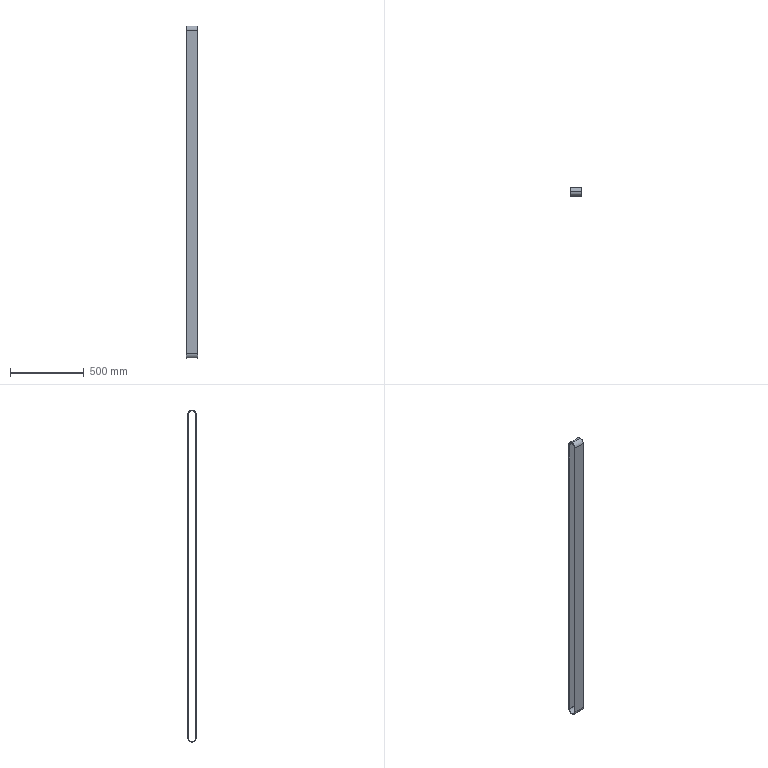Part | SolidWorks | features BossThin 1, ExtruThin 1 | 2 solids | 24 faces | box 80 x 59.15 x 2252 mm | volume 1851098 mm3 | cylinder 12 | plane 12 | commonest cylinder face diameters 54.65 x6 48.99 x3 59.15 x3
STEP:
#1=CARTESIAN_POINT('',(40.,27.325,0.));
#2=VERTEX_POINT('',#1);
#3=CARTESIAN_POINT('',(40.,0.,27.325));
#4=VERTEX_POINT('',#3);
#5=CARTESIAN_POINT('',(40.,0.,0.));
#6=DIRECTION('',(1.,0.,0.));
#7=DIRECTION('',(0.,0.,-1.));
#8=AXIS2_PLACEMENT_3D('',#5,#6,#7);
#9=CIRCLE('',#8,27.325);
#10=EDGE_CURVE('',#2,#4,#9,.T.);
#11=ORIENTED_EDGE('',*,*,#10,.T.);
#12=CARTESIAN_POINT('',(-40.,0.,27.325));
#13=VERTEX_POINT('',#12);
#14=CARTESIAN_POINT('',(40.,0.,27.325));
#15=DIRECTION('',(-1.,0.,0.));
#16=VECTOR('',#15,1000.);
#17=LINE('',#14,#16);
#18=EDGE_CURVE('',#4,#13,#17,.T.);
#19=ORIENTED_EDGE('',*,*,#18,.T.);
#20=CARTESIAN_POINT('',(-40.,27.325,0.));
#21=VERTEX_POINT('',#20);
#22=CARTESIAN_POINT('',(-40.,0.,0.));
#23=DIRECTION('',(1.,0.,0.));
#24=DIRECTION('',(0.,0.,-1.));
#25=AXIS2_PLACEMENT_3D('',#22,#23,#24);
#26=CIRCLE('',#25,27.325);
#27=EDGE_CURVE('',#21,#13,#26,.T.);
#28=ORIENTED_EDGE('',*,*,#27,.F.);
#29=CARTESIAN_POINT('',(40.,27.325,0.));
#30=DIRECTION('',(-1.,0.,0.));
#31=VECTOR('',#30,1000.);
#32=LINE('',#29,#31);
#33=EDGE_CURVE('',#2,#21,#32,.T.);
#34=ORIENTED_EDGE('',*,*,#33,.F.);
#35=EDGE_LOOP('',(#11,#19,#28,#34));
#36=FACE_OUTER_BOUND('',#35,.T.);
#37=CARTESIAN_POINT('',(40.,0.,0.));
#38=DIRECTION('',(-1.,0.,0.));
#39=DIRECTION('',(0.,0.,1.));
#40=AXIS2_PLACEMENT_3D('',#37,#38,#39);
#41=CYLINDRICAL_SURFACE('',#40,27.325);
#42=ADVANCED_FACE('',(#36),#41,.F.);
#43=CARTESIAN_POINT('',(40.,0.,29.575));
#44=VERTEX_POINT('',#43);
#45=CARTESIAN_POINT('',(40.,-29.575,0.));
#46=VERTEX_POINT('',#45);
#47=CARTESIAN_POINT('',(40.,0.,0.));
#48=DIRECTION('',(1.,0.,0.));
#49=DIRECTION('',(0.,0.,-1.));
#50=AXIS2_PLACEMENT_3D('',#47,#48,#49);
#51=CIRCLE('',#50,29.575);
#52=EDGE_CURVE('',#44,#46,#51,.T.);
#53=ORIENTED_EDGE('',*,*,#52,.F.);
#54=CARTESIAN_POINT('',(-40.,0.,29.575));
#55=VERTEX_POINT('',#54);
#56=CARTESIAN_POINT('',(40.,0.,29.575));
#57=DIRECTION('',(-1.,0.,0.));
#58=VECTOR('',#57,1000.);
#59=LINE('',#56,#58);
#60=EDGE_CURVE('',#44,#55,#59,.T.);
#61=ORIENTED_EDGE('',*,*,#60,.T.);
#62=CARTESIAN_POINT('',(-40.,-29.575,0.));
#63=VERTEX_POINT('',#62);
#64=CARTESIAN_POINT('',(-40.,0.,0.));
#65=DIRECTION('',(1.,0.,0.));
#66=DIRECTION('',(0.,0.,-1.));
#67=AXIS2_PLACEMENT_3D('',#64,#65,#66);
#68=CIRCLE('',#67,29.575);
#69=EDGE_CURVE('',#55,#63,#68,.T.);
#70=ORIENTED_EDGE('',*,*,#69,.T.);
#71=CARTESIAN_POINT('',(40.,-29.575,0.));
#72=DIRECTION('',(-1.,0.,0.));
#73=VECTOR('',#72,1000.);
#74=LINE('',#71,#73);
#75=EDGE_CURVE('',#46,#63,#74,.T.);
#76=ORIENTED_EDGE('',*,*,#75,.F.);
#77=EDGE_LOOP('',(#53,#61,#70,#76));
#78=FACE_OUTER_BOUND('',#77,.T.);
#79=CARTESIAN_POINT('',(40.,0.,0.));
#80=DIRECTION('',(-1.,0.,0.));
#81=DIRECTION('',(0.,0.,1.));
#82=AXIS2_PLACEMENT_3D('',#79,#80,#81);
#83=CYLINDRICAL_SURFACE('',#82,29.575);
#84=ADVANCED_FACE('',(#78),#83,.T.);
#85=CARTESIAN_POINT('',(40.,29.575,0.));
#86=VERTEX_POINT('',#85);
#87=CARTESIAN_POINT('',(40.,0.,0.));
#88=DIRECTION('',(1.,0.,0.));
#89=DIRECTION('',(0.,0.,-1.));
#90=AXIS2_PLACEMENT_3D('',#87,#88,#89);
#91=CIRCLE('',#90,29.575);
#92=EDGE_CURVE('',#86,#44,#91,.T.);
#93=ORIENTED_EDGE('',*,*,#92,.T.);
#94=ORIENTED_EDGE('',*,*,#52,.T.);
#95=CARTESIAN_POINT('',(40.,-29.575,-2192.5));
#96=VERTEX_POINT('',#95);
#97=CARTESIAN_POINT('',(40.,-29.575,0.));
#98=DIRECTION('',(0.,0.,-1.));
#99=VECTOR('',#98,1000.);
#100=LINE('',#97,#99);
#101=EDGE_CURVE('',#46,#96,#100,.T.);
#102=ORIENTED_EDGE('',*,*,#101,.T.);
#103=CARTESIAN_POINT('',(40.,29.575,-2192.5));
#104=VERTEX_POINT('',#103);
#105=CARTESIAN_POINT('',(40.,0.,-2192.5));
#106=DIRECTION('',(1.,0.,0.));
#107=DIRECTION('',(0.,0.,-1.));
#108=AXIS2_PLACEMENT_3D('',#105,#106,#107);
#109=CIRCLE('',#108,29.575);
#110=EDGE_CURVE('',#96,#104,#109,.T.);
#111=ORIENTED_EDGE('',*,*,#110,.T.);
#112=CARTESIAN_POINT('',(40.,29.575,0.));
#113=DIRECTION('',(0.,0.,1.));
#114=VECTOR('',#113,1000.);
#115=LINE('',#112,#114);
#116=EDGE_CURVE('',#104,#86,#115,.T.);
#117=ORIENTED_EDGE('',*,*,#116,.T.);
#118=EDGE_LOOP('',(#93,#94,#102,#111,#117));
#119=FACE_OUTER_BOUND('',#118,.T.);
#120=CARTESIAN_POINT('',(40.,-27.325,0.));
#121=VERTEX_POINT('',#120);
#122=CARTESIAN_POINT('',(40.,-27.325,-2192.5));
#123=VERTEX_POINT('',#122);
#124=CARTESIAN_POINT('',(40.,-27.325,0.));
#125=DIRECTION('',(0.,0.,-1.));
#126=VECTOR('',#125,1000.);
#127=LINE('',#124,#126);
#128=EDGE_CURVE('',#121,#123,#127,.T.);
#129=ORIENTED_EDGE('',*,*,#128,.F.);
#130=CARTESIAN_POINT('',(40.,0.,0.));
#131=DIRECTION('',(1.,0.,0.));
#132=DIRECTION('',(0.,0.,-1.));
#133=AXIS2_PLACEMENT_3D('',#130,#131,#132);
#134=CIRCLE('',#133,27.325);
#135=EDGE_CURVE('',#4,#121,#134,.T.);
#136=ORIENTED_EDGE('',*,*,#135,.F.);
#137=ORIENTED_EDGE('',*,*,#10,.F.);
#138=CARTESIAN_POINT('',(40.,27.325,-2192.5));
#139=VERTEX_POINT('',#138);
#140=CARTESIAN_POINT('',(40.,27.325,0.));
#141=DIRECTION('',(0.,0.,1.));
#142=VECTOR('',#141,1000.);
#143=LINE('',#140,#142);
#144=EDGE_CURVE('',#139,#2,#143,.T.);
#145=ORIENTED_EDGE('',*,*,#144,.F.);
#146=CARTESIAN_POINT('',(40.,0.,-2192.5));
#147=DIRECTION('',(1.,0.,0.));
#148=DIRECTION('',(0.,0.,-1.));
#149=AXIS2_PLACEMENT_3D('',#146,#147,#148);
#150=CIRCLE('',#149,27.325);
#151=EDGE_CURVE('',#123,#139,#150,.T.);
#152=ORIENTED_EDGE('',*,*,#151,.F.);
#153=EDGE_LOOP('',(#129,#136,#137,#145,#152));
#154=FACE_BOUND('',#153,.T.);
#155=CARTESIAN_POINT('',(40.,0.,0.));
#156=DIRECTION('',(1.,0.,0.));
#157=DIRECTION('',(0.,0.,-1.));
#158=AXIS2_PLACEMENT_3D('',#155,#156,#157);
#159=PLANE('',#158);
#160=ADVANCED_FACE('',(#119,#154),#159,.T.);
#161=CARTESIAN_POINT('',(-40.,29.575,0.));
#162=VERTEX_POINT('',#161);
#163=CARTESIAN_POINT('',(-40.,0.,0.));
#164=DIRECTION('',(1.,0.,0.));
#165=DIRECTION('',(0.,0.,-1.));
#166=AXIS2_PLACEMENT_3D('',#163,#164,#165);
#167=CIRCLE('',#166,29.575);
#168=EDGE_CURVE('',#162,#55,#167,.T.);
#169=ORIENTED_EDGE('',*,*,#168,.F.);
#170=CARTESIAN_POINT('',(-40.,29.575,-2192.5));
#171=VERTEX_POINT('',#170);
#172=CARTESIAN_POINT('',(-40.,29.575,0.));
#173=DIRECTION('',(0.,0.,1.));
#174=VECTOR('',#173,1000.);
#175=LINE('',#172,#174);
#176=EDGE_CURVE('',#171,#162,#175,.T.);
#177=ORIENTED_EDGE('',*,*,#176,.F.);
#178=CARTESIAN_POINT('',(-40.,-29.575,-2192.5));
#179=VERTEX_POINT('',#178);
#180=CARTESIAN_POINT('',(-40.,0.,-2192.5));
#181=DIRECTION('',(1.,0.,0.));
#182=DIRECTION('',(0.,0.,-1.));
#183=AXIS2_PLACEMENT_3D('',#180,#181,#182);
#184=CIRCLE('',#183,29.575);
#185=EDGE_CURVE('',#179,#171,#184,.T.);
#186=ORIENTED_EDGE('',*,*,#185,.F.);
#187=CARTESIAN_POINT('',(-40.,-29.575,0.));
#188=DIRECTION('',(0.,0.,-1.));
#189=VECTOR('',#188,1000.);
#190=LINE('',#187,#189);
#191=EDGE_CURVE('',#63,#179,#190,.T.);
#192=ORIENTED_EDGE('',*,*,#191,.F.);
#193=ORIENTED_EDGE('',*,*,#69,.F.);
#194=EDGE_LOOP('',(#169,#177,#186,#192,#193));
#195=FACE_OUTER_BOUND('',#194,.T.);
#196=ORIENTED_EDGE('',*,*,#27,.T.);
#197=CARTESIAN_POINT('',(-40.,-27.325,0.));
#198=VERTEX_POINT('',#197);
#199=CARTESIAN_POINT('',(-40.,0.,0.));
#200=DIRECTION('',(1.,0.,0.));
#201=DIRECTION('',(0.,0.,-1.));
#202=AXIS2_PLACEMENT_3D('',#199,#200,#201);
#203=CIRCLE('',#202,27.325);
#204=EDGE_CURVE('',#13,#198,#203,.T.);
#205=ORIENTED_EDGE('',*,*,#204,.T.);
#206=CARTESIAN_POINT('',(-40.,-27.325,-2192.5));
#207=VERTEX_POINT('',#206);
#208=CARTESIAN_POINT('',(-40.,-27.325,0.));
#209=DIRECTION('',(0.,0.,-1.));
#210=VECTOR('',#209,1000.);
#211=LINE('',#208,#210);
#212=EDGE_CURVE('',#198,#207,#211,.T.);
#213=ORIENTED_EDGE('',*,*,#212,.T.);
#214=CARTESIAN_POINT('',(-40.,27.325,-2192.5));
#215=VERTEX_POINT('',#214);
#216=CARTESIAN_POINT('',(-40.,0.,-2192.5));
#217=DIRECTION('',(1.,0.,0.));
#218=DIRECTION('',(0.,0.,-1.));
#219=AXIS2_PLACEMENT_3D('',#216,#217,#218);
#220=CIRCLE('',#219,27.325);
#221=EDGE_CURVE('',#207,#215,#220,.T.);
#222=ORIENTED_EDGE('',*,*,#221,.T.);
#223=CARTESIAN_POINT('',(-40.,27.325,0.));
#224=DIRECTION('',(0.,0.,1.));
#225=VECTOR('',#224,1000.);
#226=LINE('',#223,#225);
#227=EDGE_CURVE('',#215,#21,#226,.T.);
#228=ORIENTED_EDGE('',*,*,#227,.T.);
#229=EDGE_LOOP('',(#196,#205,#213,#222,#228));
#230=FACE_BOUND('',#229,.T.);
#231=CARTESIAN_POINT('',(-40.,0.,0.));
#232=DIRECTION('',(1.,0.,0.));
#233=DIRECTION('',(0.,0.,-1.));
#234=AXIS2_PLACEMENT_3D('',#231,#232,#233);
#235=PLANE('',#234);
#236=ADVANCED_FACE('',(#195,#230),#235,.F.);
#237=ORIENTED_EDGE('',*,*,#60,.F.);
#238=ORIENTED_EDGE('',*,*,#92,.F.);
#239=CARTESIAN_POINT('',(40.,29.575,0.));
#240=DIRECTION('',(-1.,0.,0.));
#241=VECTOR('',#240,1000.);
#242=LINE('',#239,#241);
#243=EDGE_CURVE('',#86,#162,#242,.T.);
#244=ORIENTED_EDGE('',*,*,#243,.T.);
#245=ORIENTED_EDGE('',*,*,#168,.T.);
#246=EDGE_LOOP('',(#237,#238,#244,#245));
#247=FACE_OUTER_BOUND('',#246,.T.);
#248=CARTESIAN_POINT('',(40.,0.,0.));
#249=DIRECTION('',(-1.,0.,0.));
#250=DIRECTION('',(0.,0.,1.));
#251=AXIS2_PLACEMENT_3D('',#248,#249,#250);
#252=CYLINDRICAL_SURFACE('',#251,29.575);
#253=ADVANCED_FACE('',(#247),#252,.T.);
#254=ORIENTED_EDGE('',*,*,#191,.T.);
#255=CARTESIAN_POINT('',(40.,-29.575,-2192.5));
#256=DIRECTION('',(-1.,0.,0.));
#257=VECTOR('',#256,1000.);
#258=LINE('',#255,#257);
#259=EDGE_CURVE('',#96,#179,#258,.T.);
#260=ORIENTED_EDGE('',*,*,#259,.F.);
#261=ORIENTED_EDGE('',*,*,#101,.F.);
#262=ORIENTED_EDGE('',*,*,#75,.T.);
#263=EDGE_LOOP('',(#254,#260,#261,#262));
#264=FACE_OUTER_BOUND('',#263,.T.);
#265=CARTESIAN_POINT('',(40.,-29.575,0.));
#266=DIRECTION('',(0.,1.,0.));
#267=DIRECTION('',(0.,0.,1.));
#268=AXIS2_PLACEMENT_3D('',#265,#266,#267);
#269=PLANE('',#268);
#270=ADVANCED_FACE('',(#264),#269,.F.);
#271=ORIENTED_EDGE('',*,*,#185,.T.);
#272=CARTESIAN_POINT('',(40.,29.575,-2192.5));
#273=DIRECTION('',(-1.,0.,0.));
#274=VECTOR('',#273,1000.);
#275=LINE('',#272,#274);
#276=EDGE_CURVE('',#104,#171,#275,.T.);
#277=ORIENTED_EDGE('',*,*,#276,.F.);
#278=ORIENTED_EDGE('',*,*,#110,.F.);
#279=ORIENTED_EDGE('',*,*,#259,.T.);
#280=EDGE_LOOP('',(#271,#277,#278,#279));
#281=FACE_OUTER_BOUND('',#280,.T.);
#282=CARTESIAN_POINT('',(40.,0.,-2192.5));
#283=DIRECTION('',(-1.,0.,0.));
#284=DIRECTION('',(0.,0.,1.));
#285=AXIS2_PLACEMENT_3D('',#282,#283,#284);
#286=CYLINDRICAL_SURFACE('',#285,29.575);
#287=ADVANCED_FACE('',(#281),#286,.T.);
#288=ORIENTED_EDGE('',*,*,#176,.T.);
#289=ORIENTED_EDGE('',*,*,#243,.F.);
#290=ORIENTED_EDGE('',*,*,#116,.F.);
#291=ORIENTED_EDGE('',*,*,#276,.T.);
#292=EDGE_LOOP('',(#288,#289,#290,#291));
#293=FACE_OUTER_BOUND('',#292,.T.);
#294=CARTESIAN_POINT('',(40.,29.575,0.));
#295=DIRECTION('',(0.,-1.,0.));
#296=DIRECTION('',(0.,0.,-1.));
#297=AXIS2_PLACEMENT_3D('',#294,#295,#296);
#298=PLANE('',#297);
#299=ADVANCED_FACE('',(#293),#298,.F.);
#300=ORIENTED_EDGE('',*,*,#18,.F.);
#301=ORIENTED_EDGE('',*,*,#135,.T.);
#302=CARTESIAN_POINT('',(40.,-27.325,0.));
#303=DIRECTION('',(-1.,0.,0.));
#304=VECTOR('',#303,1000.);
#305=LINE('',#302,#304);
#306=EDGE_CURVE('',#121,#198,#305,.T.);
#307=ORIENTED_EDGE('',*,*,#306,.T.);
#308=ORIENTED_EDGE('',*,*,#204,.F.);
#309=EDGE_LOOP('',(#300,#301,#307,#308));
#310=FACE_OUTER_BOUND('',#309,.T.);
#311=CARTESIAN_POINT('',(40.,0.,0.));
#312=DIRECTION('',(-1.,0.,0.));
#313=DIRECTION('',(0.,0.,1.));
#314=AXIS2_PLACEMENT_3D('',#311,#312,#313);
#315=CYLINDRICAL_SURFACE('',#314,27.325);
#316=ADVANCED_FACE('',(#310),#315,.F.);
#317=ORIENTED_EDGE('',*,*,#212,.F.);
#318=ORIENTED_EDGE('',*,*,#306,.F.);
#319=ORIENTED_EDGE('',*,*,#128,.T.);
#320=CARTESIAN_POINT('',(40.,-27.325,-2192.5));
#321=DIRECTION('',(-1.,0.,0.));
#322=VECTOR('',#321,1000.);
#323=LINE('',#320,#322);
#324=EDGE_CURVE('',#123,#207,#323,.T.);
#325=ORIENTED_EDGE('',*,*,#324,.T.);
#326=EDGE_LOOP('',(#317,#318,#319,#325));
#327=FACE_OUTER_BOUND('',#326,.T.);
#328=CARTESIAN_POINT('',(40.,-27.325,0.));
#329=DIRECTION('',(0.,1.,0.));
#330=DIRECTION('',(0.,0.,1.));
#331=AXIS2_PLACEMENT_3D('',#328,#329,#330);
#332=PLANE('',#331);
#333=ADVANCED_FACE('',(#327),#332,.T.);
#334=ORIENTED_EDGE('',*,*,#221,.F.);
#335=ORIENTED_EDGE('',*,*,#324,.F.);
#336=ORIENTED_EDGE('',*,*,#151,.T.);
#337=CARTESIAN_POINT('',(40.,27.325,-2192.5));
#338=DIRECTION('',(-1.,0.,0.));
#339=VECTOR('',#338,1000.);
#340=LINE('',#337,#339);
#341=EDGE_CURVE('',#139,#215,#340,.T.);
#342=ORIENTED_EDGE('',*,*,#341,.T.);
#343=EDGE_LOOP('',(#334,#335,#336,#342));
#344=FACE_OUTER_BOUND('',#343,.T.);
#345=CARTESIAN_POINT('',(40.,0.,-2192.5));
#346=DIRECTION('',(-1.,0.,0.));
#347=DIRECTION('',(0.,0.,1.));
#348=AXIS2_PLACEMENT_3D('',#345,#346,#347);
#349=CYLINDRICAL_SURFACE('',#348,27.325);
#350=ADVANCED_FACE('',(#344),#349,.F.);
#351=ORIENTED_EDGE('',*,*,#227,.F.);
#352=ORIENTED_EDGE('',*,*,#341,.F.);
#353=ORIENTED_EDGE('',*,*,#144,.T.);
#354=ORIENTED_EDGE('',*,*,#33,.T.);
#355=EDGE_LOOP('',(#351,#352,#353,#354));
#356=FACE_OUTER_BOUND('',#355,.T.);
#357=CARTESIAN_POINT('',(40.,27.325,0.));
#358=DIRECTION('',(0.,-1.,0.));
#359=DIRECTION('',(0.,0.,-1.));
#360=AXIS2_PLACEMENT_3D('',#357,#358,#359);
#361=PLANE('',#360);
#362=ADVANCED_FACE('',(#356),#361,.T.);
#363=CLOSED_SHELL('',(#42,#84,#160,#236,#253,#270,#287,#299,#316,#333,#350,#362));
#364=MANIFOLD_SOLID_BREP('',#363);
#365=CARTESIAN_POINT('',(40.,24.495,0.));
#366=VERTEX_POINT('',#365);
#367=CARTESIAN_POINT('',(40.,0.,24.495));
#368=VERTEX_POINT('',#367);
#369=CARTESIAN_POINT('',(40.,0.,0.));
#370=DIRECTION('',(1.,0.,0.));
#371=DIRECTION('',(0.,0.,-1.));
#372=AXIS2_PLACEMENT_3D('',#369,#370,#371);
#373=CIRCLE('',#372,24.495);
#374=EDGE_CURVE('',#366,#368,#373,.T.);
#375=ORIENTED_EDGE('',*,*,#374,.T.);
#376=CARTESIAN_POINT('',(-40.,0.,24.495));
#377=VERTEX_POINT('',#376);
#378=CARTESIAN_POINT('',(40.,0.,24.495));
#379=DIRECTION('',(-1.,0.,0.));
#380=VECTOR('',#379,1000.);
#381=LINE('',#378,#380);
#382=EDGE_CURVE('',#368,#377,#381,.T.);
#383=ORIENTED_EDGE('',*,*,#382,.T.);
#384=CARTESIAN_POINT('',(-40.,24.495,0.));
#385=VERTEX_POINT('',#384);
#386=CARTESIAN_POINT('',(-40.,0.,0.));
#387=DIRECTION('',(1.,0.,0.));
#388=DIRECTION('',(0.,0.,-1.));
#389=AXIS2_PLACEMENT_3D('',#386,#387,#388);
#390=CIRCLE('',#389,24.495);
#391=EDGE_CURVE('',#385,#377,#390,.T.);
#392=ORIENTED_EDGE('',*,*,#391,.F.);
#393=CARTESIAN_POINT('',(40.,24.495,0.));
#394=DIRECTION('',(-1.,0.,0.));
#395=VECTOR('',#394,1000.);
#396=LINE('',#393,#395);
#397=EDGE_CURVE('',#366,#385,#396,.T.);
#398=ORIENTED_EDGE('',*,*,#397,.F.);
#399=EDGE_LOOP('',(#375,#383,#392,#398));
#400=FACE_OUTER_BOUND('',#399,.T.);
#401=CARTESIAN_POINT('',(40.,0.,0.));
#402=DIRECTION('',(-1.,0.,0.));
#403=DIRECTION('',(0.,0.,1.));
#404=AXIS2_PLACEMENT_3D('',#401,#402,#403);
#405=CYLINDRICAL_SURFACE('',#404,24.495);
#406=ADVANCED_FACE('',(#400),#405,.F.);
#407=CARTESIAN_POINT('',(40.,0.,27.325));
#408=VERTEX_POINT('',#407);
#409=CARTESIAN_POINT('',(40.,-27.325,0.));
#410=VERTEX_POINT('',#409);
#411=CARTESIAN_POINT('',(40.,0.,0.));
#412=DIRECTION('',(1.,0.,0.));
#413=DIRECTION('',(0.,0.,-1.));
#414=AXIS2_PLACEMENT_3D('',#411,#412,#413);
#415=CIRCLE('',#414,27.325);
#416=EDGE_CURVE('',#408,#410,#415,.T.);
#417=ORIENTED_EDGE('',*,*,#416,.F.);
#418=CARTESIAN_POINT('',(-40.,0.,27.325));
#419=VERTEX_POINT('',#418);
#420=CARTESIAN_POINT('',(40.,0.,27.325));
#421=DIRECTION('',(-1.,0.,0.));
#422=VECTOR('',#421,1000.);
#423=LINE('',#420,#422);
#424=EDGE_CURVE('',#408,#419,#423,.T.);
#425=ORIENTED_EDGE('',*,*,#424,.T.);
#426=CARTESIAN_POINT('',(-40.,-27.325,0.));
#427=VERTEX_POINT('',#426);
#428=CARTESIAN_POINT('',(-40.,0.,0.));
#429=DIRECTION('',(1.,0.,0.));
#430=DIRECTION('',(0.,0.,-1.));
#431=AXIS2_PLACEMENT_3D('',#428,#429,#430);
#432=CIRCLE('',#431,27.325);
#433=EDGE_CURVE('',#419,#427,#432,.T.);
#434=ORIENTED_EDGE('',*,*,#433,.T.);
#435=CARTESIAN_POINT('',(40.,-27.325,0.));
#436=DIRECTION('',(-1.,0.,0.));
#437=VECTOR('',#436,1000.);
#438=LINE('',#435,#437);
#439=EDGE_CURVE('',#410,#427,#438,.T.);
#440=ORIENTED_EDGE('',*,*,#439,.F.);
#441=EDGE_LOOP('',(#417,#425,#434,#440));
#442=FACE_OUTER_BOUND('',#441,.T.);
#443=CARTESIAN_POINT('',(40.,0.,0.));
#444=DIRECTION('',(-1.,0.,0.));
#445=DIRECTION('',(0.,0.,1.));
#446=AXIS2_PLACEMENT_3D('',#443,#444,#445);
#447=CYLINDRICAL_SURFACE('',#446,27.325);
#448=ADVANCED_FACE('',(#442),#447,.T.);
#449=CARTESIAN_POINT('',(40.,27.325,0.));
#450=VERTEX_POINT('',#449);
#451=CARTESIAN_POINT('',(40.,0.,0.));
#452=DIRECTION('',(1.,0.,0.));
#453=DIRECTION('',(0.,0.,-1.));
#454=AXIS2_PLACEMENT_3D('',#451,#452,#453);
#455=CIRCLE('',#454,27.325);
#456=EDGE_CURVE('',#450,#408,#455,.T.);
#457=ORIENTED_EDGE('',*,*,#456,.T.);
#458=ORIENTED_EDGE('',*,*,#416,.T.);
#459=CARTESIAN_POINT('',(40.,-27.325,-2192.5));
#460=VERTEX_POINT('',#459);
#461=CARTESIAN_POINT('',(40.,-27.325,0.));
#462=DIRECTION('',(0.,0.,-1.));
#463=VECTOR('',#462,1000.);
#464=LINE('',#461,#463);
#465=EDGE_CURVE('',#410,#460,#464,.T.);
#466=ORIENTED_EDGE('',*,*,#465,.T.);
#467=CARTESIAN_POINT('',(40.,27.325,-2192.5));
#468=VERTEX_POINT('',#467);
#469=CARTESIAN_POINT('',(40.,0.,-2192.5));
#470=DIRECTION('',(1.,0.,0.));
#471=DIRECTION('',(0.,0.,-1.));
#472=AXIS2_PLACEMENT_3D('',#469,#470,#471);
#473=CIRCLE('',#472,27.325);
#474=EDGE_CURVE('',#460,#468,#473,.T.);
#475=ORIENTED_EDGE('',*,*,#474,.T.);
#476=CARTESIAN_POINT('',(40.,27.325,-2192.5));
#477=DIRECTION('',(0.,0.,1.));
#478=VECTOR('',#477,1000.);
#479=LINE('',#476,#478);
#480=EDGE_CURVE('',#468,#450,#479,.T.);
#481=ORIENTED_EDGE('',*,*,#480,.T.);
#482=EDGE_LOOP('',(#457,#458,#466,#475,#481));
#483=FACE_OUTER_BOUND('',#482,.T.);
#484=CARTESIAN_POINT('',(40.,-24.495,0.));
#485=VERTEX_POINT('',#484);
#486=CARTESIAN_POINT('',(40.,-24.495,-2192.5));
#487=VERTEX_POINT('',#486);
#488=CARTESIAN_POINT('',(40.,-24.495,0.));
#489=DIRECTION('',(0.,0.,-1.));
#490=VECTOR('',#489,1000.);
#491=LINE('',#488,#490);
#492=EDGE_CURVE('',#485,#487,#491,.T.);
#493=ORIENTED_EDGE('',*,*,#492,.F.);
#494=CARTESIAN_POINT('',(40.,0.,0.));
#495=DIRECTION('',(1.,0.,0.));
#496=DIRECTION('',(0.,0.,-1.));
#497=AXIS2_PLACEMENT_3D('',#494,#495,#496);
#498=CIRCLE('',#497,24.495);
#499=EDGE_CURVE('',#368,#485,#498,.T.);
#500=ORIENTED_EDGE('',*,*,#499,.F.);
#501=ORIENTED_EDGE('',*,*,#374,.F.);
#502=CARTESIAN_POINT('',(40.,24.495,-2192.5));
#503=VERTEX_POINT('',#502);
#504=CARTESIAN_POINT('',(40.,24.495,-2192.5));
#505=DIRECTION('',(0.,0.,1.));
#506=VECTOR('',#505,1000.);
#507=LINE('',#504,#506);
#508=EDGE_CURVE('',#503,#366,#507,.T.);
#509=ORIENTED_EDGE('',*,*,#508,.F.);
#510=CARTESIAN_POINT('',(40.,0.,-2192.5));
#511=DIRECTION('',(1.,0.,0.));
#512=DIRECTION('',(0.,0.,-1.));
#513=AXIS2_PLACEMENT_3D('',#510,#511,#512);
#514=CIRCLE('',#513,24.495);
#515=EDGE_CURVE('',#487,#503,#514,.T.);
#516=ORIENTED_EDGE('',*,*,#515,.F.);
#517=EDGE_LOOP('',(#493,#500,#501,#509,#516));
#518=FACE_BOUND('',#517,.T.);
#519=CARTESIAN_POINT('',(40.,0.,0.));
#520=DIRECTION('',(1.,0.,0.));
#521=DIRECTION('',(0.,0.,-1.));
#522=AXIS2_PLACEMENT_3D('',#519,#520,#521);
#523=PLANE('',#522);
#524=ADVANCED_FACE('',(#483,#518),#523,.T.);
#525=CARTESIAN_POINT('',(-40.,27.325,0.));
#526=VERTEX_POINT('',#525);
#527=CARTESIAN_POINT('',(-40.,0.,0.));
#528=DIRECTION('',(1.,0.,0.));
#529=DIRECTION('',(0.,0.,-1.));
#530=AXIS2_PLACEMENT_3D('',#527,#528,#529);
#531=CIRCLE('',#530,27.325);
#532=EDGE_CURVE('',#526,#419,#531,.T.);
#533=ORIENTED_EDGE('',*,*,#532,.F.);
#534=CARTESIAN_POINT('',(-40.,27.325,-2192.5));
#535=VERTEX_POINT('',#534);
#536=CARTESIAN_POINT('',(-40.,27.325,-2192.5));
#537=DIRECTION('',(0.,0.,1.));
#538=VECTOR('',#537,1000.);
#539=LINE('',#536,#538);
#540=EDGE_CURVE('',#535,#526,#539,.T.);
#541=ORIENTED_EDGE('',*,*,#540,.F.);
#542=CARTESIAN_POINT('',(-40.,-27.325,-2192.5));
#543=VERTEX_POINT('',#542);
#544=CARTESIAN_POINT('',(-40.,0.,-2192.5));
#545=DIRECTION('',(1.,0.,0.));
#546=DIRECTION('',(0.,0.,-1.));
#547=AXIS2_PLACEMENT_3D('',#544,#545,#546);
#548=CIRCLE('',#547,27.325);
#549=EDGE_CURVE('',#543,#535,#548,.T.);
#550=ORIENTED_EDGE('',*,*,#549,.F.);
#551=CARTESIAN_POINT('',(-40.,-27.325,0.));
#552=DIRECTION('',(0.,0.,-1.));
#553=VECTOR('',#552,1000.);
#554=LINE('',#551,#553);
#555=EDGE_CURVE('',#427,#543,#554,.T.);
#556=ORIENTED_EDGE('',*,*,#555,.F.);
#557=ORIENTED_EDGE('',*,*,#433,.F.);
#558=EDGE_LOOP('',(#533,#541,#550,#556,#557));
#559=FACE_OUTER_BOUND('',#558,.T.);
#560=ORIENTED_EDGE('',*,*,#391,.T.);
#561=CARTESIAN_POINT('',(-40.,-24.495,0.));
#562=VERTEX_POINT('',#561);
#563=CARTESIAN_POINT('',(-40.,0.,0.));
#564=DIRECTION('',(1.,0.,0.));
#565=DIRECTION('',(0.,0.,-1.));
#566=AXIS2_PLACEMENT_3D('',#563,#564,#565);
#567=CIRCLE('',#566,24.495);
#568=EDGE_CURVE('',#377,#562,#567,.T.);
#569=ORIENTED_EDGE('',*,*,#568,.T.);
#570=CARTESIAN_POINT('',(-40.,-24.495,-2192.5));
#571=VERTEX_POINT('',#570);
#572=CARTESIAN_POINT('',(-40.,-24.495,0.));
#573=DIRECTION('',(0.,0.,-1.));
#574=VECTOR('',#573,1000.);
#575=LINE('',#572,#574);
#576=EDGE_CURVE('',#562,#571,#575,.T.);
#577=ORIENTED_EDGE('',*,*,#576,.T.);
#578=CARTESIAN_POINT('',(-40.,24.495,-2192.5));
#579=VERTEX_POINT('',#578);
#580=CARTESIAN_POINT('',(-40.,0.,-2192.5));
#581=DIRECTION('',(1.,0.,0.));
#582=DIRECTION('',(0.,0.,-1.));
#583=AXIS2_PLACEMENT_3D('',#580,#581,#582);
#584=CIRCLE('',#583,24.495);
#585=EDGE_CURVE('',#571,#579,#584,.T.);
#586=ORIENTED_EDGE('',*,*,#585,.T.);
#587=CARTESIAN_POINT('',(-40.,24.495,-2192.5));
#588=DIRECTION('',(0.,0.,1.));
#589=VECTOR('',#588,1000.);
#590=LINE('',#587,#589);
#591=EDGE_CURVE('',#579,#385,#590,.T.);
#592=ORIENTED_EDGE('',*,*,#591,.T.);
#593=EDGE_LOOP('',(#560,#569,#577,#586,#592));
#594=FACE_BOUND('',#593,.T.);
#595=CARTESIAN_POINT('',(-40.,0.,0.));
#596=DIRECTION('',(1.,0.,0.));
#597=DIRECTION('',(0.,0.,-1.));
#598=AXIS2_PLACEMENT_3D('',#595,#596,#597);
#599=PLANE('',#598);
#600=ADVANCED_FACE('',(#559,#594),#599,.F.);
#601=ORIENTED_EDGE('',*,*,#424,.F.);
#602=ORIENTED_EDGE('',*,*,#456,.F.);
#603=CARTESIAN_POINT('',(40.,27.325,0.));
#604=DIRECTION('',(-1.,0.,0.));
#605=VECTOR('',#604,1000.);
#606=LINE('',#603,#605);
#607=EDGE_CURVE('',#450,#526,#606,.T.);
#608=ORIENTED_EDGE('',*,*,#607,.T.);
#609=ORIENTED_EDGE('',*,*,#532,.T.);
#610=EDGE_LOOP('',(#601,#602,#608,#609));
#611=FACE_OUTER_BOUND('',#610,.T.);
#612=CARTESIAN_POINT('',(40.,0.,0.));
#613=DIRECTION('',(-1.,0.,0.));
#614=DIRECTION('',(0.,0.,1.));
#615=AXIS2_PLACEMENT_3D('',#612,#613,#614);
#616=CYLINDRICAL_SURFACE('',#615,27.325);
#617=ADVANCED_FACE('',(#611),#616,.T.);
#618=ORIENTED_EDGE('',*,*,#555,.T.);
#619=CARTESIAN_POINT('',(40.,-27.325,-2192.5));
#620=DIRECTION('',(-1.,0.,0.));
#621=VECTOR('',#620,1000.);
#622=LINE('',#619,#621);
#623=EDGE_CURVE('',#460,#543,#622,.T.);
#624=ORIENTED_EDGE('',*,*,#623,.F.);
#625=ORIENTED_EDGE('',*,*,#465,.F.);
#626=ORIENTED_EDGE('',*,*,#439,.T.);
#627=EDGE_LOOP('',(#618,#624,#625,#626));
#628=FACE_OUTER_BOUND('',#627,.T.);
#629=CARTESIAN_POINT('',(40.,-27.325,0.));
#630=DIRECTION('',(0.,1.,0.));
#631=DIRECTION('',(0.,0.,1.));
#632=AXIS2_PLACEMENT_3D('',#629,#630,#631);
#633=PLANE('',#632);
#634=ADVANCED_FACE('',(#628),#633,.F.);
#635=ORIENTED_EDGE('',*,*,#549,.T.);
#636=CARTESIAN_POINT('',(40.,27.325,-2192.5));
#637=DIRECTION('',(-1.,0.,0.));
#638=VECTOR('',#637,1000.);
#639=LINE('',#636,#638);
#640=EDGE_CURVE('',#468,#535,#639,.T.);
#641=ORIENTED_EDGE('',*,*,#640,.F.);
#642=ORIENTED_EDGE('',*,*,#474,.F.);
#643=ORIENTED_EDGE('',*,*,#623,.T.);
#644=EDGE_LOOP('',(#635,#641,#642,#643));
#645=FACE_OUTER_BOUND('',#644,.T.);
#646=CARTESIAN_POINT('',(40.,0.,-2192.5));
#647=DIRECTION('',(-1.,0.,0.));
#648=DIRECTION('',(0.,0.,1.));
#649=AXIS2_PLACEMENT_3D('',#646,#647,#648);
#650=CYLINDRICAL_SURFACE('',#649,27.325);
#651=ADVANCED_FACE('',(#645),#650,.T.);
#652=ORIENTED_EDGE('',*,*,#540,.T.);
#653=ORIENTED_EDGE('',*,*,#607,.F.);
#654=ORIENTED_EDGE('',*,*,#480,.F.);
#655=ORIENTED_EDGE('',*,*,#640,.T.);
#656=EDGE_LOOP('',(#652,#653,#654,#655));
#657=FACE_OUTER_BOUND('',#656,.T.);
#658=CARTESIAN_POINT('',(40.,27.325,-2192.5));
#659=DIRECTION('',(0.,-1.,0.));
#660=DIRECTION('',(0.,0.,-1.));
#661=AXIS2_PLACEMENT_3D('',#658,#659,#660);
#662=PLANE('',#661);
#663=ADVANCED_FACE('',(#657),#662,.F.);
#664=ORIENTED_EDGE('',*,*,#382,.F.);
#665=ORIENTED_EDGE('',*,*,#499,.T.);
#666=CARTESIAN_POINT('',(40.,-24.495,0.));
#667=DIRECTION('',(-1.,0.,0.));
#668=VECTOR('',#667,1000.);
#669=LINE('',#666,#668);
#670=EDGE_CURVE('',#485,#562,#669,.T.);
#671=ORIENTED_EDGE('',*,*,#670,.T.);
#672=ORIENTED_EDGE('',*,*,#568,.F.);
#673=EDGE_LOOP('',(#664,#665,#671,#672));
#674=FACE_OUTER_BOUND('',#673,.T.);
#675=CARTESIAN_POINT('',(40.,0.,0.));
#676=DIRECTION('',(-1.,0.,0.));
#677=DIRECTION('',(0.,0.,1.));
#678=AXIS2_PLACEMENT_3D('',#675,#676,#677);
#679=CYLINDRICAL_SURFACE('',#678,24.495);
#680=ADVANCED_FACE('',(#674),#679,.F.);
#681=ORIENTED_EDGE('',*,*,#576,.F.);
#682=ORIENTED_EDGE('',*,*,#670,.F.);
#683=ORIENTED_EDGE('',*,*,#492,.T.);
#684=CARTESIAN_POINT('',(40.,-24.495,-2192.5));
#685=DIRECTION('',(-1.,0.,0.));
#686=VECTOR('',#685,1000.);
#687=LINE('',#684,#686);
#688=EDGE_CURVE('',#487,#571,#687,.T.);
#689=ORIENTED_EDGE('',*,*,#688,.T.);
#690=EDGE_LOOP('',(#681,#682,#683,#689));
#691=FACE_OUTER_BOUND('',#690,.T.);
#692=CARTESIAN_POINT('',(40.,-24.495,0.));
#693=DIRECTION('',(0.,1.,0.));
#694=DIRECTION('',(0.,0.,1.));
#695=AXIS2_PLACEMENT_3D('',#692,#693,#694);
#696=PLANE('',#695);
#697=ADVANCED_FACE('',(#691),#696,.T.);
#698=ORIENTED_EDGE('',*,*,#585,.F.);
#699=ORIENTED_EDGE('',*,*,#688,.F.);
#700=ORIENTED_EDGE('',*,*,#515,.T.);
#701=CARTESIAN_POINT('',(40.,24.495,-2192.5));
#702=DIRECTION('',(-1.,0.,0.));
#703=VECTOR('',#702,1000.);
#704=LINE('',#701,#703);
#705=EDGE_CURVE('',#503,#579,#704,.T.);
#706=ORIENTED_EDGE('',*,*,#705,.T.);
#707=EDGE_LOOP('',(#698,#699,#700,#706));
#708=FACE_OUTER_BOUND('',#707,.T.);
#709=CARTESIAN_POINT('',(40.,0.,-2192.5));
#710=DIRECTION('',(-1.,0.,0.));
#711=DIRECTION('',(0.,0.,1.));
#712=AXIS2_PLACEMENT_3D('',#709,#710,#711);
#713=CYLINDRICAL_SURFACE('',#712,24.495);
#714=ADVANCED_FACE('',(#708),#713,.F.);
#715=ORIENTED_EDGE('',*,*,#591,.F.);
#716=ORIENTED_EDGE('',*,*,#705,.F.);
#717=ORIENTED_EDGE('',*,*,#508,.T.);
#718=ORIENTED_EDGE('',*,*,#397,.T.);
#719=EDGE_LOOP('',(#715,#716,#717,#718));
#720=FACE_OUTER_BOUND('',#719,.T.);
#721=CARTESIAN_POINT('',(40.,24.495,-2192.5));
#722=DIRECTION('',(0.,-1.,0.));
#723=DIRECTION('',(0.,0.,-1.));
#724=AXIS2_PLACEMENT_3D('',#721,#722,#723);
#725=PLANE('',#724);
#726=ADVANCED_FACE('',(#720),#725,.T.);
#727=CLOSED_SHELL('',(#406,#448,#524,#600,#617,#634,#651,#663,#680,#697,#714,#726));
#728=MANIFOLD_SOLID_BREP('',#727);
#729=CARTESIAN_POINT('',(0.,0.,0.));
#730=DIRECTION('',(0.,0.,1.));
#731=DIRECTION('',(1.,0.,0.));
#732=AXIS2_PLACEMENT_3D('',#729,#730,#731);
#733=(LENGTH_UNIT()NAMED_UNIT(*)SI_UNIT(.MILLI.,.METRE.));
#734=UNCERTAINTY_MEASURE_WITH_UNIT(LENGTH_MEASURE(0.00001),#733,'','');
#735=(NAMED_UNIT(*)PLANE_ANGLE_UNIT()SI_UNIT($,.RADIAN.));
#736=(NAMED_UNIT(*)SI_UNIT($,.STERADIAN.)SOLID_ANGLE_UNIT());
#737=(GEOMETRIC_REPRESENTATION_CONTEXT(3)GLOBAL_UNCERTAINTY_ASSIGNED_CONTEXT((#734))GLOBAL_UNIT_ASSIGNED_CONTEXT((#733,#735,#736))REPRESENTATION_CONTEXT('',''));
#738=ADVANCED_BREP_SHAPE_REPRESENTATION('',(#364,#728,#732),#737);